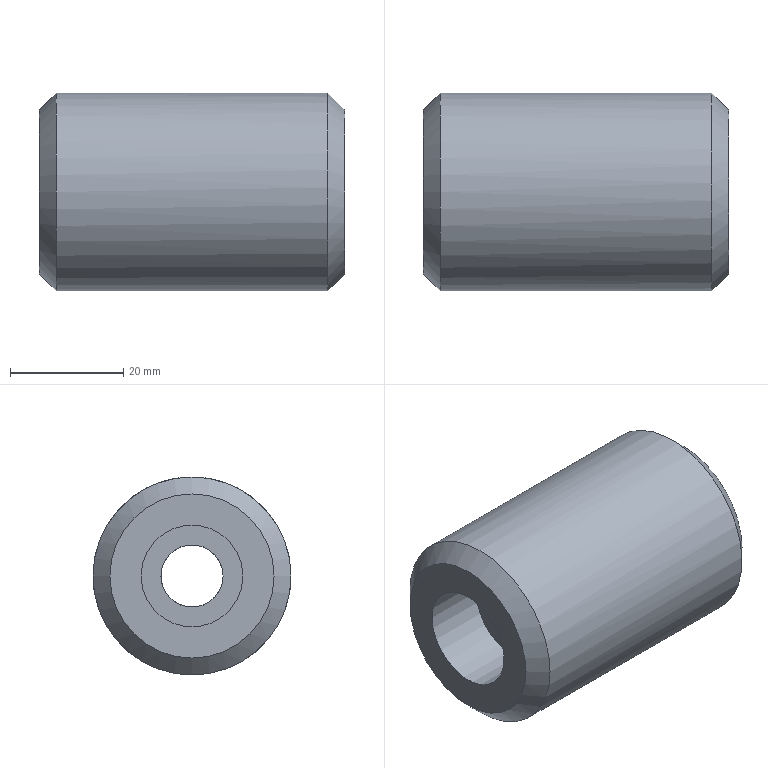Part | STEP file | solid 69 | 1 solid | 8 faces | box 54 x 35 x 35 mm | volume 44135 mm3 | plane 3 | cylinder 3 | cone 2 | commonest cylinder face diameters 11 x1 18 x1 35 x1